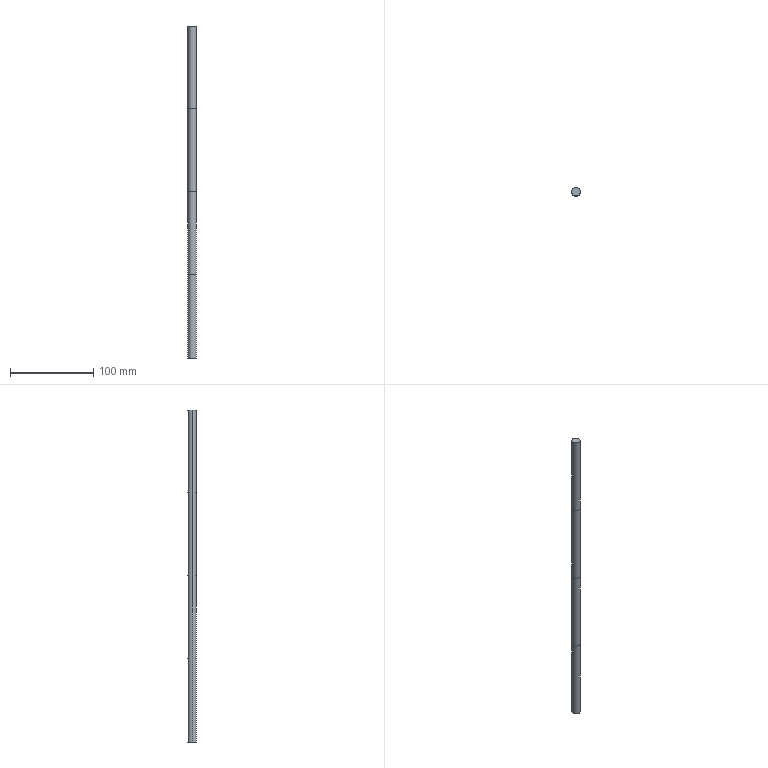Part | SolidWorks | features Extrusion 1, PLine 1 | 1 solid | 10 faces | box 10 x 10 x 400 mm | volume 31416 mm3 | cylinder 8 | plane 2 | commonest cylinder face diameters 10 x8
STEP:
#1=CARTESIAN_POINT('',(-5.,0.,100.));
#2=VERTEX_POINT('',#1);
#3=CARTESIAN_POINT('',(5.,0.,100.));
#4=VERTEX_POINT('',#3);
#5=CARTESIAN_POINT('',(0.,0.,100.));
#6=DIRECTION('',(0.,0.,-1.));
#7=DIRECTION('',(-1.,0.,0.));
#8=AXIS2_PLACEMENT_3D('',#5,#6,#7);
#9=CIRCLE('',#8,5.);
#10=EDGE_CURVE('',#2,#4,#9,.T.);
#11=ORIENTED_EDGE('',*,*,#10,.T.);
#12=CARTESIAN_POINT('',(5.,0.,0.));
#13=VERTEX_POINT('',#12);
#14=CARTESIAN_POINT('',(5.,0.,400.));
#15=DIRECTION('',(0.,0.,-1.));
#16=VECTOR('',#15,1000.);
#17=LINE('',#14,#16);
#18=EDGE_CURVE('',#4,#13,#17,.T.);
#19=ORIENTED_EDGE('',*,*,#18,.T.);
#20=CARTESIAN_POINT('',(-5.,0.,0.));
#21=VERTEX_POINT('',#20);
#22=CARTESIAN_POINT('',(0.,0.,0.));
#23=DIRECTION('',(0.,0.,1.));
#24=DIRECTION('',(1.,0.,0.));
#25=AXIS2_PLACEMENT_3D('',#22,#23,#24);
#26=CIRCLE('',#25,5.);
#27=EDGE_CURVE('',#13,#21,#26,.T.);
#28=ORIENTED_EDGE('',*,*,#27,.T.);
#29=CARTESIAN_POINT('',(-5.,0.,400.));
#30=DIRECTION('',(0.,0.,-1.));
#31=VECTOR('',#30,1000.);
#32=LINE('',#29,#31);
#33=EDGE_CURVE('',#2,#21,#32,.T.);
#34=ORIENTED_EDGE('',*,*,#33,.F.);
#35=EDGE_LOOP('',(#11,#19,#28,#34));
#36=FACE_OUTER_BOUND('',#35,.T.);
#37=CARTESIAN_POINT('',(0.,0.,400.));
#38=DIRECTION('',(0.,0.,-1.));
#39=DIRECTION('',(-1.,0.,0.));
#40=AXIS2_PLACEMENT_3D('',#37,#38,#39);
#41=CYLINDRICAL_SURFACE('',#40,5.);
#42=ADVANCED_FACE('',(#36),#41,.T.);
#43=CARTESIAN_POINT('',(5.,0.,400.));
#44=VERTEX_POINT('',#43);
#45=CARTESIAN_POINT('',(-5.,0.,400.));
#46=VERTEX_POINT('',#45);
#47=CARTESIAN_POINT('',(0.,0.,400.));
#48=DIRECTION('',(0.,0.,1.));
#49=DIRECTION('',(1.,0.,0.));
#50=AXIS2_PLACEMENT_3D('',#47,#48,#49);
#51=CIRCLE('',#50,5.);
#52=EDGE_CURVE('',#44,#46,#51,.T.);
#53=ORIENTED_EDGE('',*,*,#52,.F.);
#54=CARTESIAN_POINT('',(5.,0.,300.));
#55=VERTEX_POINT('',#54);
#56=CARTESIAN_POINT('',(5.,0.,400.));
#57=DIRECTION('',(0.,0.,-1.));
#58=VECTOR('',#57,1000.);
#59=LINE('',#56,#58);
#60=EDGE_CURVE('',#44,#55,#59,.T.);
#61=ORIENTED_EDGE('',*,*,#60,.T.);
#62=CARTESIAN_POINT('',(-5.,0.,300.));
#63=VERTEX_POINT('',#62);
#64=CARTESIAN_POINT('',(0.,0.,300.));
#65=DIRECTION('',(0.,0.,-1.));
#66=DIRECTION('',(-1.,0.,0.));
#67=AXIS2_PLACEMENT_3D('',#64,#65,#66);
#68=CIRCLE('',#67,5.);
#69=EDGE_CURVE('',#63,#55,#68,.T.);
#70=ORIENTED_EDGE('',*,*,#69,.F.);
#71=CARTESIAN_POINT('',(-5.,0.,400.));
#72=DIRECTION('',(0.,0.,-1.));
#73=VECTOR('',#72,1000.);
#74=LINE('',#71,#73);
#75=EDGE_CURVE('',#46,#63,#74,.T.);
#76=ORIENTED_EDGE('',*,*,#75,.F.);
#77=EDGE_LOOP('',(#53,#61,#70,#76));
#78=FACE_OUTER_BOUND('',#77,.T.);
#79=CARTESIAN_POINT('',(0.,0.,400.));
#80=DIRECTION('',(0.,0.,-1.));
#81=DIRECTION('',(-1.,0.,0.));
#82=AXIS2_PLACEMENT_3D('',#79,#80,#81);
#83=CYLINDRICAL_SURFACE('',#82,5.);
#84=ADVANCED_FACE('',(#78),#83,.T.);
#85=ORIENTED_EDGE('',*,*,#69,.T.);
#86=CARTESIAN_POINT('',(5.,0.,200.));
#87=VERTEX_POINT('',#86);
#88=CARTESIAN_POINT('',(5.,0.,400.));
#89=DIRECTION('',(0.,0.,-1.));
#90=VECTOR('',#89,1000.);
#91=LINE('',#88,#90);
#92=EDGE_CURVE('',#55,#87,#91,.T.);
#93=ORIENTED_EDGE('',*,*,#92,.T.);
#94=CARTESIAN_POINT('',(-5.,0.,200.));
#95=VERTEX_POINT('',#94);
#96=CARTESIAN_POINT('',(0.,0.,200.));
#97=DIRECTION('',(0.,0.,-1.));
#98=DIRECTION('',(-1.,0.,0.));
#99=AXIS2_PLACEMENT_3D('',#96,#97,#98);
#100=CIRCLE('',#99,5.);
#101=EDGE_CURVE('',#95,#87,#100,.T.);
#102=ORIENTED_EDGE('',*,*,#101,.F.);
#103=CARTESIAN_POINT('',(-5.,0.,400.));
#104=DIRECTION('',(0.,0.,-1.));
#105=VECTOR('',#104,1000.);
#106=LINE('',#103,#105);
#107=EDGE_CURVE('',#63,#95,#106,.T.);
#108=ORIENTED_EDGE('',*,*,#107,.F.);
#109=EDGE_LOOP('',(#85,#93,#102,#108));
#110=FACE_OUTER_BOUND('',#109,.T.);
#111=CARTESIAN_POINT('',(0.,0.,400.));
#112=DIRECTION('',(0.,0.,-1.));
#113=DIRECTION('',(-1.,0.,0.));
#114=AXIS2_PLACEMENT_3D('',#111,#112,#113);
#115=CYLINDRICAL_SURFACE('',#114,5.);
#116=ADVANCED_FACE('',(#110),#115,.T.);
#117=ORIENTED_EDGE('',*,*,#101,.T.);
#118=CARTESIAN_POINT('',(5.,0.,400.));
#119=DIRECTION('',(0.,0.,-1.));
#120=VECTOR('',#119,1000.);
#121=LINE('',#118,#120);
#122=EDGE_CURVE('',#87,#4,#121,.T.);
#123=ORIENTED_EDGE('',*,*,#122,.T.);
#124=ORIENTED_EDGE('',*,*,#10,.F.);
#125=CARTESIAN_POINT('',(-5.,0.,400.));
#126=DIRECTION('',(0.,0.,-1.));
#127=VECTOR('',#126,1000.);
#128=LINE('',#125,#127);
#129=EDGE_CURVE('',#95,#2,#128,.T.);
#130=ORIENTED_EDGE('',*,*,#129,.F.);
#131=EDGE_LOOP('',(#117,#123,#124,#130));
#132=FACE_OUTER_BOUND('',#131,.T.);
#133=CARTESIAN_POINT('',(0.,0.,400.));
#134=DIRECTION('',(0.,0.,-1.));
#135=DIRECTION('',(-1.,0.,0.));
#136=AXIS2_PLACEMENT_3D('',#133,#134,#135);
#137=CYLINDRICAL_SURFACE('',#136,5.);
#138=ADVANCED_FACE('',(#132),#137,.T.);
#139=ORIENTED_EDGE('',*,*,#122,.F.);
#140=CARTESIAN_POINT('',(0.,0.,200.));
#141=DIRECTION('',(0.,0.,-1.));
#142=DIRECTION('',(-1.,0.,0.));
#143=AXIS2_PLACEMENT_3D('',#140,#141,#142);
#144=CIRCLE('',#143,5.);
#145=EDGE_CURVE('',#87,#95,#144,.T.);
#146=ORIENTED_EDGE('',*,*,#145,.T.);
#147=ORIENTED_EDGE('',*,*,#129,.T.);
#148=CARTESIAN_POINT('',(0.,0.,100.));
#149=DIRECTION('',(0.,0.,-1.));
#150=DIRECTION('',(-1.,0.,0.));
#151=AXIS2_PLACEMENT_3D('',#148,#149,#150);
#152=CIRCLE('',#151,5.);
#153=EDGE_CURVE('',#4,#2,#152,.T.);
#154=ORIENTED_EDGE('',*,*,#153,.F.);
#155=EDGE_LOOP('',(#139,#146,#147,#154));
#156=FACE_OUTER_BOUND('',#155,.T.);
#157=CARTESIAN_POINT('',(0.,0.,400.));
#158=DIRECTION('',(0.,0.,-1.));
#159=DIRECTION('',(-1.,0.,0.));
#160=AXIS2_PLACEMENT_3D('',#157,#158,#159);
#161=CYLINDRICAL_SURFACE('',#160,5.);
#162=ADVANCED_FACE('',(#156),#161,.T.);
#163=ORIENTED_EDGE('',*,*,#92,.F.);
#164=CARTESIAN_POINT('',(0.,0.,300.));
#165=DIRECTION('',(0.,0.,-1.));
#166=DIRECTION('',(-1.,0.,0.));
#167=AXIS2_PLACEMENT_3D('',#164,#165,#166);
#168=CIRCLE('',#167,5.);
#169=EDGE_CURVE('',#55,#63,#168,.T.);
#170=ORIENTED_EDGE('',*,*,#169,.T.);
#171=ORIENTED_EDGE('',*,*,#107,.T.);
#172=ORIENTED_EDGE('',*,*,#145,.F.);
#173=EDGE_LOOP('',(#163,#170,#171,#172));
#174=FACE_OUTER_BOUND('',#173,.T.);
#175=CARTESIAN_POINT('',(0.,0.,400.));
#176=DIRECTION('',(0.,0.,-1.));
#177=DIRECTION('',(-1.,0.,0.));
#178=AXIS2_PLACEMENT_3D('',#175,#176,#177);
#179=CYLINDRICAL_SURFACE('',#178,5.);
#180=ADVANCED_FACE('',(#174),#179,.T.);
#181=ORIENTED_EDGE('',*,*,#60,.F.);
#182=CARTESIAN_POINT('',(0.,0.,400.));
#183=DIRECTION('',(0.,0.,1.));
#184=DIRECTION('',(1.,0.,0.));
#185=AXIS2_PLACEMENT_3D('',#182,#183,#184);
#186=CIRCLE('',#185,5.);
#187=EDGE_CURVE('',#46,#44,#186,.T.);
#188=ORIENTED_EDGE('',*,*,#187,.F.);
#189=ORIENTED_EDGE('',*,*,#75,.T.);
#190=ORIENTED_EDGE('',*,*,#169,.F.);
#191=EDGE_LOOP('',(#181,#188,#189,#190));
#192=FACE_OUTER_BOUND('',#191,.T.);
#193=CARTESIAN_POINT('',(0.,0.,400.));
#194=DIRECTION('',(0.,0.,-1.));
#195=DIRECTION('',(-1.,0.,0.));
#196=AXIS2_PLACEMENT_3D('',#193,#194,#195);
#197=CYLINDRICAL_SURFACE('',#196,5.);
#198=ADVANCED_FACE('',(#192),#197,.T.);
#199=ORIENTED_EDGE('',*,*,#18,.F.);
#200=ORIENTED_EDGE('',*,*,#153,.T.);
#201=ORIENTED_EDGE('',*,*,#33,.T.);
#202=CARTESIAN_POINT('',(0.,0.,0.));
#203=DIRECTION('',(0.,0.,1.));
#204=DIRECTION('',(1.,0.,0.));
#205=AXIS2_PLACEMENT_3D('',#202,#203,#204);
#206=CIRCLE('',#205,5.);
#207=EDGE_CURVE('',#21,#13,#206,.T.);
#208=ORIENTED_EDGE('',*,*,#207,.T.);
#209=EDGE_LOOP('',(#199,#200,#201,#208));
#210=FACE_OUTER_BOUND('',#209,.T.);
#211=CARTESIAN_POINT('',(0.,0.,400.));
#212=DIRECTION('',(0.,0.,-1.));
#213=DIRECTION('',(-1.,0.,0.));
#214=AXIS2_PLACEMENT_3D('',#211,#212,#213);
#215=CYLINDRICAL_SURFACE('',#214,5.);
#216=ADVANCED_FACE('',(#210),#215,.T.);
#217=ORIENTED_EDGE('',*,*,#187,.T.);
#218=ORIENTED_EDGE('',*,*,#52,.T.);
#219=EDGE_LOOP('',(#217,#218));
#220=FACE_OUTER_BOUND('',#219,.T.);
#221=CARTESIAN_POINT('',(0.,0.,400.));
#222=DIRECTION('',(0.,0.,1.));
#223=DIRECTION('',(1.,0.,0.));
#224=AXIS2_PLACEMENT_3D('',#221,#222,#223);
#225=PLANE('',#224);
#226=ADVANCED_FACE('',(#220),#225,.T.);
#227=ORIENTED_EDGE('',*,*,#207,.F.);
#228=ORIENTED_EDGE('',*,*,#27,.F.);
#229=EDGE_LOOP('',(#227,#228));
#230=FACE_OUTER_BOUND('',#229,.T.);
#231=CARTESIAN_POINT('',(0.,0.,0.));
#232=DIRECTION('',(0.,0.,1.));
#233=DIRECTION('',(1.,0.,0.));
#234=AXIS2_PLACEMENT_3D('',#231,#232,#233);
#235=PLANE('',#234);
#236=ADVANCED_FACE('',(#230),#235,.F.);
#237=CLOSED_SHELL('',(#42,#84,#116,#138,#162,#180,#198,#216,#226,#236));
#238=MANIFOLD_SOLID_BREP('',#237);
#239=CARTESIAN_POINT('',(0.,0.,0.));
#240=DIRECTION('',(0.,0.,1.));
#241=DIRECTION('',(1.,0.,0.));
#242=AXIS2_PLACEMENT_3D('',#239,#240,#241);
#243=(LENGTH_UNIT()NAMED_UNIT(*)SI_UNIT(.MILLI.,.METRE.));
#244=UNCERTAINTY_MEASURE_WITH_UNIT(LENGTH_MEASURE(0.00001),#243,'','');
#245=(NAMED_UNIT(*)PLANE_ANGLE_UNIT()SI_UNIT($,.RADIAN.));
#246=(NAMED_UNIT(*)SI_UNIT($,.STERADIAN.)SOLID_ANGLE_UNIT());
#247=(GEOMETRIC_REPRESENTATION_CONTEXT(3)GLOBAL_UNCERTAINTY_ASSIGNED_CONTEXT((#244))GLOBAL_UNIT_ASSIGNED_CONTEXT((#243,#245,#246))REPRESENTATION_CONTEXT('',''));
#248=ADVANCED_BREP_SHAPE_REPRESENTATION('',(#238,#242),#247);